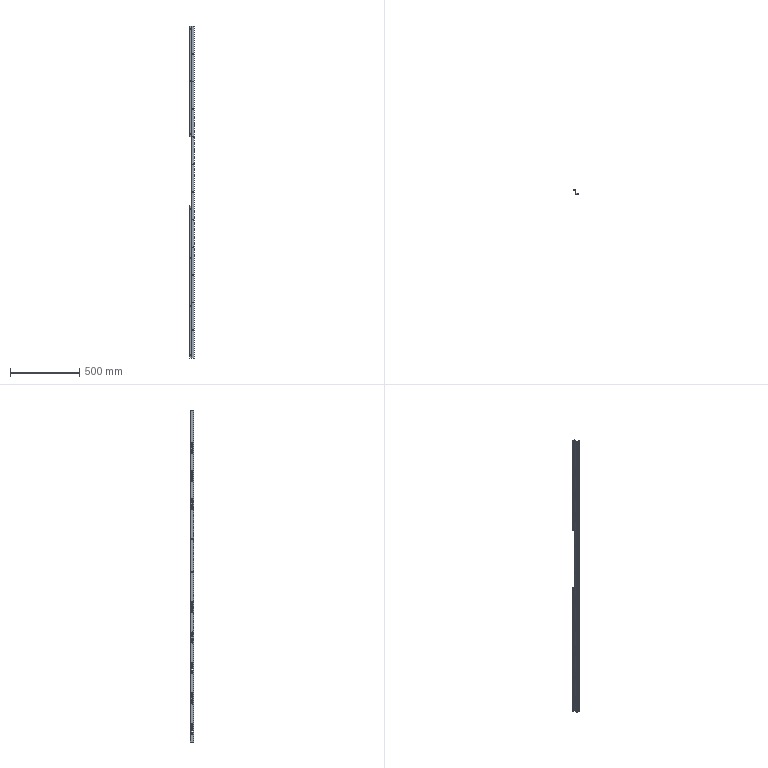Part | SolidWorks | features ICE 6, LPattern 2, EdgeFlange 1, FlatPattern 1, SMBaseFlange 1, SheetMetal 1 | 1 solid | 144 faces | box 33.5 x 28 x 2396 mm | volume 191583 mm3 | cylinder 80 | plane 64 | commonest cylinder face diameters 7 x38 5 x25 6.2 x14 2 x3